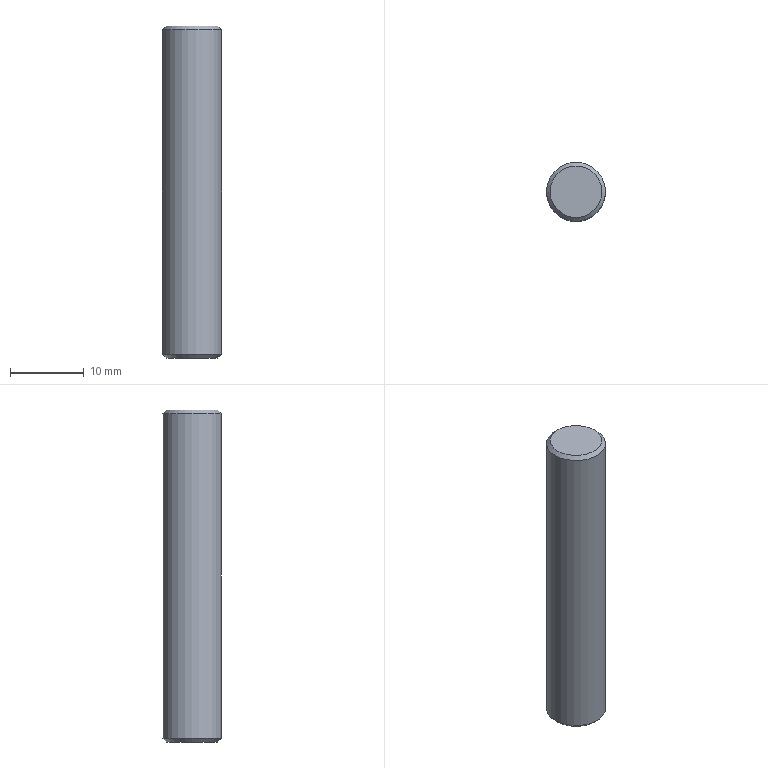Part | NX | features DATUM_CSYS 2, CHAMFER 1, EXTRUDE 1, SKETCH 1 | 1 solid | 5 faces | box 8 x 8 x 45 mm | volume 2256 mm3 | plane 2 | cone 2 | cylinder 1 | commonest cylinder face diameters 8 x1
STEP:
#1=CARTESIAN_POINT('',(4.,0.,0.5));
#2=VERTEX_POINT('',#1);
#3=CARTESIAN_POINT('',(0.,0.,0.5));
#4=DIRECTION('',(0.,0.,1.));
#5=DIRECTION('',(1.,0.,0.));
#6=AXIS2_PLACEMENT_3D('',#3,#4,#5);
#7=CIRCLE('',#6,4.);
#8=EDGE_CURVE('',#2,#2,#7,.T.);
#9=ORIENTED_EDGE('',*,*,#8,.T.);
#10=EDGE_LOOP('',(#9));
#11=FACE_BOUND('',#10,.T.);
#12=CARTESIAN_POINT('',(4.,0.,44.5));
#13=VERTEX_POINT('',#12);
#14=CARTESIAN_POINT('',(0.,0.,44.5));
#15=DIRECTION('',(0.,0.,1.));
#16=DIRECTION('',(1.,0.,0.));
#17=AXIS2_PLACEMENT_3D('',#14,#15,#16);
#18=CIRCLE('',#17,4.);
#19=EDGE_CURVE('',#13,#13,#18,.F.);
#20=ORIENTED_EDGE('',*,*,#19,.T.);
#21=EDGE_LOOP('',(#20));
#22=FACE_BOUND('',#21,.T.);
#23=CARTESIAN_POINT('',(0.,0.,45.));
#24=DIRECTION('',(0.,0.,-1.));
#25=DIRECTION('',(-1.,0.,0.));
#26=AXIS2_PLACEMENT_3D('',#23,#24,#25);
#27=CYLINDRICAL_SURFACE('',#26,4.);
#28=ADVANCED_FACE('',(#11,#22),#27,.T.);
#29=CARTESIAN_POINT('',(3.5,0.,45.));
#30=VERTEX_POINT('',#29);
#31=CARTESIAN_POINT('',(0.,0.,45.));
#32=DIRECTION('',(0.,0.,1.));
#33=DIRECTION('',(1.,0.,0.));
#34=AXIS2_PLACEMENT_3D('',#31,#32,#33);
#35=CIRCLE('',#34,3.5);
#36=EDGE_CURVE('',#30,#30,#35,.T.);
#37=ORIENTED_EDGE('',*,*,#36,.T.);
#38=EDGE_LOOP('',(#37));
#39=FACE_BOUND('',#38,.T.);
#40=CARTESIAN_POINT('',(0.,0.,45.));
#41=DIRECTION('',(0.,0.,1.));
#42=DIRECTION('',(1.,0.,0.));
#43=AXIS2_PLACEMENT_3D('',#40,#41,#42);
#44=PLANE('',#43);
#45=ADVANCED_FACE('',(#39),#44,.T.);
#46=CARTESIAN_POINT('',(3.5,0.,0.));
#47=VERTEX_POINT('',#46);
#48=CARTESIAN_POINT('',(0.,0.,0.));
#49=DIRECTION('',(0.,0.,1.));
#50=DIRECTION('',(1.,0.,0.));
#51=AXIS2_PLACEMENT_3D('',#48,#49,#50);
#52=CIRCLE('',#51,3.5);
#53=EDGE_CURVE('',#47,#47,#52,.F.);
#54=ORIENTED_EDGE('',*,*,#53,.T.);
#55=EDGE_LOOP('',(#54));
#56=FACE_BOUND('',#55,.T.);
#57=CARTESIAN_POINT('',(0.,0.,0.));
#58=DIRECTION('',(0.,0.,1.));
#59=DIRECTION('',(1.,0.,0.));
#60=AXIS2_PLACEMENT_3D('',#57,#58,#59);
#61=PLANE('',#60);
#62=ADVANCED_FACE('',(#56),#61,.F.);
#63=ORIENTED_EDGE('',*,*,#53,.F.);
#64=EDGE_LOOP('',(#63));
#65=FACE_BOUND('',#64,.T.);
#66=ORIENTED_EDGE('',*,*,#8,.F.);
#67=EDGE_LOOP('',(#66));
#68=FACE_BOUND('',#67,.T.);
#69=CARTESIAN_POINT('',(0.,0.,0.5));
#70=DIRECTION('',(0.,0.,1.));
#71=DIRECTION('',(1.,0.,0.));
#72=AXIS2_PLACEMENT_3D('',#69,#70,#71);
#73=CONICAL_SURFACE('',#72,4.,0.7854);
#74=ADVANCED_FACE('',(#65,#68),#73,.T.);
#75=ORIENTED_EDGE('',*,*,#19,.F.);
#76=EDGE_LOOP('',(#75));
#77=FACE_BOUND('',#76,.T.);
#78=ORIENTED_EDGE('',*,*,#36,.F.);
#79=EDGE_LOOP('',(#78));
#80=FACE_BOUND('',#79,.T.);
#81=CARTESIAN_POINT('',(0.,0.,45.));
#82=DIRECTION('',(0.,0.,-1.));
#83=DIRECTION('',(-1.,0.,0.));
#84=AXIS2_PLACEMENT_3D('',#81,#82,#83);
#85=CONICAL_SURFACE('',#84,3.5,0.7854);
#86=ADVANCED_FACE('',(#77,#80),#85,.T.);
#87=CLOSED_SHELL('',(#28,#45,#62,#74,#86));
#88=MANIFOLD_SOLID_BREP('',#87);
#89=(LENGTH_UNIT()NAMED_UNIT(*)SI_UNIT(.MILLI.,.METRE.));
#90=UNCERTAINTY_MEASURE_WITH_UNIT(LENGTH_MEASURE(0.00001),#89,'','');
#91=(NAMED_UNIT(*)PLANE_ANGLE_UNIT()SI_UNIT($,.RADIAN.));
#92=(NAMED_UNIT(*)SI_UNIT($,.STERADIAN.)SOLID_ANGLE_UNIT());
#93=(GEOMETRIC_REPRESENTATION_CONTEXT(3)GLOBAL_UNCERTAINTY_ASSIGNED_CONTEXT((#90))GLOBAL_UNIT_ASSIGNED_CONTEXT((#89,#91,#92))REPRESENTATION_CONTEXT('',''));
#94=ADVANCED_BREP_SHAPE_REPRESENTATION('',(#88),#93);